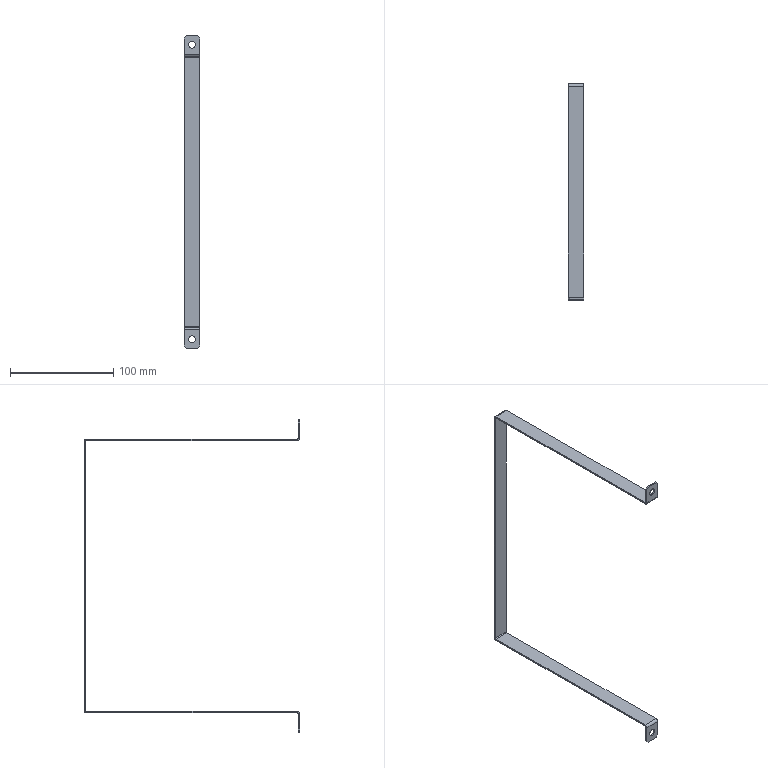Part | SolidWorks | features BaseBody 1 | 1 solid | 30 faces | box 15 x 208.5 x 302 mm | volume 15925 mm3 | plane 18 | cylinder 12 | commonest cylinder face diameters 1.473 x4 4.473 x4 7 x4
STEP:
#1=CARTESIAN_POINT('',(0.,1.5,-146.));
#2=VERTEX_POINT('',#1);
#3=CARTESIAN_POINT('',(0.,1.5,-139.));
#4=VERTEX_POINT('',#3);
#5=CARTESIAN_POINT('',(0.,1.5,-142.5));
#6=DIRECTION('',(0.,1.,0.));
#7=DIRECTION('',(0.,0.,-1.));
#8=AXIS2_PLACEMENT_3D('',#5,#6,#7);
#9=CIRCLE('',#8,3.5);
#10=EDGE_CURVE('',#2,#4,#9,.T.);
#11=ORIENTED_EDGE('',*,*,#10,.T.);
#12=CARTESIAN_POINT('',(0.,0.,-139.));
#13=VERTEX_POINT('',#12);
#14=CARTESIAN_POINT('',(0.,208.501,-139.));
#15=DIRECTION('',(0.,-1.,0.));
#16=VECTOR('',#15,1000.);
#17=LINE('',#14,#16);
#18=EDGE_CURVE('',#4,#13,#17,.T.);
#19=ORIENTED_EDGE('',*,*,#18,.T.);
#20=CARTESIAN_POINT('',(0.,0.,-146.));
#21=VERTEX_POINT('',#20);
#22=CARTESIAN_POINT('',(0.,0.,-142.5));
#23=DIRECTION('',(0.,-1.,0.));
#24=DIRECTION('',(0.,0.,1.));
#25=AXIS2_PLACEMENT_3D('',#22,#23,#24);
#26=CIRCLE('',#25,3.5);
#27=EDGE_CURVE('',#13,#21,#26,.T.);
#28=ORIENTED_EDGE('',*,*,#27,.T.);
#29=CARTESIAN_POINT('',(0.,208.501,-146.));
#30=DIRECTION('',(0.,-1.,0.));
#31=VECTOR('',#30,1000.);
#32=LINE('',#29,#31);
#33=EDGE_CURVE('',#2,#21,#32,.T.);
#34=ORIENTED_EDGE('',*,*,#33,.F.);
#35=EDGE_LOOP('',(#11,#19,#28,#34));
#36=FACE_OUTER_BOUND('',#35,.T.);
#37=CARTESIAN_POINT('',(0.,208.501,-142.5));
#38=DIRECTION('',(0.,-1.,0.));
#39=DIRECTION('',(0.,0.,-1.));
#40=AXIS2_PLACEMENT_3D('',#37,#38,#39);
#41=CYLINDRICAL_SURFACE('',#40,3.5);
#42=ADVANCED_FACE('',(#36),#41,.F.);
#43=CARTESIAN_POINT('',(0.,1.5,139.));
#44=VERTEX_POINT('',#43);
#45=CARTESIAN_POINT('',(0.,1.5,146.));
#46=VERTEX_POINT('',#45);
#47=CARTESIAN_POINT('',(0.,1.5,142.5));
#48=DIRECTION('',(0.,1.,0.));
#49=DIRECTION('',(0.,0.,-1.));
#50=AXIS2_PLACEMENT_3D('',#47,#48,#49);
#51=CIRCLE('',#50,3.5);
#52=EDGE_CURVE('',#44,#46,#51,.T.);
#53=ORIENTED_EDGE('',*,*,#52,.T.);
#54=CARTESIAN_POINT('',(0.,0.,146.));
#55=VERTEX_POINT('',#54);
#56=CARTESIAN_POINT('',(0.,208.501,146.));
#57=DIRECTION('',(0.,-1.,0.));
#58=VECTOR('',#57,1000.);
#59=LINE('',#56,#58);
#60=EDGE_CURVE('',#46,#55,#59,.T.);
#61=ORIENTED_EDGE('',*,*,#60,.T.);
#62=CARTESIAN_POINT('',(0.,0.,139.));
#63=VERTEX_POINT('',#62);
#64=CARTESIAN_POINT('',(0.,0.,142.5));
#65=DIRECTION('',(0.,-1.,0.));
#66=DIRECTION('',(0.,0.,-1.));
#67=AXIS2_PLACEMENT_3D('',#64,#65,#66);
#68=CIRCLE('',#67,3.5);
#69=EDGE_CURVE('',#55,#63,#68,.T.);
#70=ORIENTED_EDGE('',*,*,#69,.T.);
#71=CARTESIAN_POINT('',(0.,208.501,139.));
#72=DIRECTION('',(0.,-1.,0.));
#73=VECTOR('',#72,1000.);
#74=LINE('',#71,#73);
#75=EDGE_CURVE('',#44,#63,#74,.T.);
#76=ORIENTED_EDGE('',*,*,#75,.F.);
#77=EDGE_LOOP('',(#53,#61,#70,#76));
#78=FACE_OUTER_BOUND('',#77,.T.);
#79=CARTESIAN_POINT('',(0.,208.501,142.5));
#80=DIRECTION('',(0.,-1.,0.));
#81=DIRECTION('',(0.,0.,-1.));
#82=AXIS2_PLACEMENT_3D('',#79,#80,#81);
#83=CYLINDRICAL_SURFACE('',#82,3.5);
#84=ADVANCED_FACE('',(#78),#83,.F.);
#85=CARTESIAN_POINT('',(-5.5,0.,151.));
#86=VERTEX_POINT('',#85);
#87=CARTESIAN_POINT('',(-7.5,0.,149.));
#88=VERTEX_POINT('',#87);
#89=CARTESIAN_POINT('',(1.,0.,157.5));
#90=DIRECTION('',(-0.7071,0.,-0.7071));
#91=VECTOR('',#90,1000.);
#92=LINE('',#89,#91);
#93=EDGE_CURVE('',#86,#88,#92,.T.);
#94=ORIENTED_EDGE('',*,*,#93,.F.);
#95=CARTESIAN_POINT('',(-5.5,1.5,151.));
#96=VERTEX_POINT('',#95);
#97=CARTESIAN_POINT('',(-5.5,0.,151.));
#98=DIRECTION('',(0.,-1.,0.));
#99=VECTOR('',#98,1000.);
#100=LINE('',#97,#99);
#101=EDGE_CURVE('',#96,#86,#100,.T.);
#102=ORIENTED_EDGE('',*,*,#101,.F.);
#103=CARTESIAN_POINT('',(-7.5,1.5,149.));
#104=VERTEX_POINT('',#103);
#105=CARTESIAN_POINT('',(-7.5,1.5,149.));
#106=DIRECTION('',(0.7071,0.,0.7071));
#107=VECTOR('',#106,1000.);
#108=LINE('',#105,#107);
#109=EDGE_CURVE('',#104,#96,#108,.T.);
#110=ORIENTED_EDGE('',*,*,#109,.F.);
#111=CARTESIAN_POINT('',(-7.5,2.237,149.));
#112=DIRECTION('',(0.,1.,0.));
#113=VECTOR('',#112,1000.);
#114=LINE('',#111,#113);
#115=EDGE_CURVE('',#88,#104,#114,.T.);
#116=ORIENTED_EDGE('',*,*,#115,.F.);
#117=EDGE_LOOP('',(#94,#102,#110,#116));
#118=FACE_OUTER_BOUND('',#117,.T.);
#119=CARTESIAN_POINT('',(-7.5,2.237,149.));
#120=DIRECTION('',(0.7071,0.,-0.7071));
#121=DIRECTION('',(0.,-1.,0.));
#122=AXIS2_PLACEMENT_3D('',#119,#120,#121);
#123=PLANE('',#122);
#124=ADVANCED_FACE('',(#118),#123,.F.);
#125=CARTESIAN_POINT('',(7.5,0.,149.));
#126=VERTEX_POINT('',#125);
#127=CARTESIAN_POINT('',(5.5,0.,151.));
#128=VERTEX_POINT('',#127);
#129=CARTESIAN_POINT('',(6.5,0.,150.));
#130=DIRECTION('',(-0.7071,0.,0.7071));
#131=VECTOR('',#130,1000.);
#132=LINE('',#129,#131);
#133=EDGE_CURVE('',#126,#128,#132,.T.);
#134=ORIENTED_EDGE('',*,*,#133,.F.);
#135=CARTESIAN_POINT('',(7.5,1.5,149.));
#136=VERTEX_POINT('',#135);
#137=CARTESIAN_POINT('',(7.5,2.237,149.));
#138=DIRECTION('',(0.,-1.,0.));
#139=VECTOR('',#138,1000.);
#140=LINE('',#137,#139);
#141=EDGE_CURVE('',#136,#126,#140,.T.);
#142=ORIENTED_EDGE('',*,*,#141,.F.);
#143=CARTESIAN_POINT('',(5.5,1.5,151.));
#144=VERTEX_POINT('',#143);
#145=CARTESIAN_POINT('',(5.5,1.5,151.));
#146=DIRECTION('',(0.7071,0.,-0.7071));
#147=VECTOR('',#146,1000.);
#148=LINE('',#145,#147);
#149=EDGE_CURVE('',#144,#136,#148,.T.);
#150=ORIENTED_EDGE('',*,*,#149,.F.);
#151=CARTESIAN_POINT('',(5.5,0.,151.));
#152=DIRECTION('',(0.,1.,0.));
#153=VECTOR('',#152,1000.);
#154=LINE('',#151,#153);
#155=EDGE_CURVE('',#128,#144,#154,.T.);
#156=ORIENTED_EDGE('',*,*,#155,.F.);
#157=EDGE_LOOP('',(#134,#142,#150,#156));
#158=FACE_OUTER_BOUND('',#157,.T.);
#159=CARTESIAN_POINT('',(5.5,0.,151.));
#160=DIRECTION('',(-0.7071,0.,-0.7071));
#161=DIRECTION('',(-0.7071,0.,0.7071));
#162=AXIS2_PLACEMENT_3D('',#159,#160,#161);
#163=PLANE('',#162);
#164=ADVANCED_FACE('',(#158),#163,.F.);
#165=CARTESIAN_POINT('',(-5.5,1.5,-151.));
#166=VERTEX_POINT('',#165);
#167=CARTESIAN_POINT('',(-7.5,1.5,-149.));
#168=VERTEX_POINT('',#167);
#169=CARTESIAN_POINT('',(-7.5,1.5,-149.));
#170=DIRECTION('',(-0.7071,0.,0.7071));
#171=VECTOR('',#170,1000.);
#172=LINE('',#169,#171);
#173=EDGE_CURVE('',#166,#168,#172,.T.);
#174=ORIENTED_EDGE('',*,*,#173,.F.);
#175=CARTESIAN_POINT('',(-5.5,0.,-151.));
#176=VERTEX_POINT('',#175);
#177=CARTESIAN_POINT('',(-5.5,1.5,-151.));
#178=DIRECTION('',(0.,1.,0.));
#179=VECTOR('',#178,1000.);
#180=LINE('',#177,#179);
#181=EDGE_CURVE('',#176,#166,#180,.T.);
#182=ORIENTED_EDGE('',*,*,#181,.F.);
#183=CARTESIAN_POINT('',(-7.5,0.,-149.));
#184=VERTEX_POINT('',#183);
#185=CARTESIAN_POINT('',(1.,0.,-157.5));
#186=DIRECTION('',(0.7071,0.,-0.7071));
#187=VECTOR('',#186,1000.);
#188=LINE('',#185,#187);
#189=EDGE_CURVE('',#184,#176,#188,.T.);
#190=ORIENTED_EDGE('',*,*,#189,.F.);
#191=CARTESIAN_POINT('',(-7.5,2.237,-149.));
#192=DIRECTION('',(0.,-1.,0.));
#193=VECTOR('',#192,1000.);
#194=LINE('',#191,#193);
#195=EDGE_CURVE('',#168,#184,#194,.T.);
#196=ORIENTED_EDGE('',*,*,#195,.F.);
#197=EDGE_LOOP('',(#174,#182,#190,#196));
#198=FACE_OUTER_BOUND('',#197,.T.);
#199=CARTESIAN_POINT('',(-7.5,2.237,-149.));
#200=DIRECTION('',(0.7071,0.,0.7071));
#201=DIRECTION('',(0.,-1.,0.));
#202=AXIS2_PLACEMENT_3D('',#199,#200,#201);
#203=PLANE('',#202);
#204=ADVANCED_FACE('',(#198),#203,.F.);
#205=CARTESIAN_POINT('',(7.5,1.5,-149.));
#206=VERTEX_POINT('',#205);
#207=CARTESIAN_POINT('',(5.5,1.5,-151.));
#208=VERTEX_POINT('',#207);
#209=CARTESIAN_POINT('',(5.5,1.5,-151.));
#210=DIRECTION('',(-0.7071,0.,-0.7071));
#211=VECTOR('',#210,1000.);
#212=LINE('',#209,#211);
#213=EDGE_CURVE('',#206,#208,#212,.T.);
#214=ORIENTED_EDGE('',*,*,#213,.F.);
#215=CARTESIAN_POINT('',(7.5,0.,-149.));
#216=VERTEX_POINT('',#215);
#217=CARTESIAN_POINT('',(7.5,1.5,-149.));
#218=DIRECTION('',(0.,1.,0.));
#219=VECTOR('',#218,1000.);
#220=LINE('',#217,#219);
#221=EDGE_CURVE('',#216,#206,#220,.T.);
#222=ORIENTED_EDGE('',*,*,#221,.F.);
#223=CARTESIAN_POINT('',(5.5,0.,-151.));
#224=VERTEX_POINT('',#223);
#225=CARTESIAN_POINT('',(6.5,0.,-150.));
#226=DIRECTION('',(0.7071,0.,0.7071));
#227=VECTOR('',#226,1000.);
#228=LINE('',#225,#227);
#229=EDGE_CURVE('',#224,#216,#228,.T.);
#230=ORIENTED_EDGE('',*,*,#229,.F.);
#231=CARTESIAN_POINT('',(5.5,0.,-151.));
#232=DIRECTION('',(0.,-1.,0.));
#233=VECTOR('',#232,1000.);
#234=LINE('',#231,#233);
#235=EDGE_CURVE('',#208,#224,#234,.T.);
#236=ORIENTED_EDGE('',*,*,#235,.F.);
#237=EDGE_LOOP('',(#214,#222,#230,#236));
#238=FACE_OUTER_BOUND('',#237,.T.);
#239=CARTESIAN_POINT('',(5.5,1.5,-151.));
#240=DIRECTION('',(0.7071,0.,-0.7071));
#241=DIRECTION('',(0.,-1.,0.));
#242=AXIS2_PLACEMENT_3D('',#239,#240,#241);
#243=PLANE('',#242);
#244=ADVANCED_FACE('',(#238),#243,.T.);
#245=CARTESIAN_POINT('',(-7.5,2.237,132.5));
#246=VERTEX_POINT('',#245);
#247=CARTESIAN_POINT('',(-7.5,1.5,133.237));
#248=VERTEX_POINT('',#247);
#249=CARTESIAN_POINT('',(-7.5,2.237,133.237));
#250=DIRECTION('',(-1.,0.,0.));
#251=DIRECTION('',(0.,0.,-1.));
#252=AXIS2_PLACEMENT_3D('',#249,#250,#251);
#253=CIRCLE('',#252,0.7366);
#254=EDGE_CURVE('',#246,#248,#253,.T.);
#255=ORIENTED_EDGE('',*,*,#254,.T.);
#256=CARTESIAN_POINT('',(7.5,1.5,133.237));
#257=VERTEX_POINT('',#256);
#258=CARTESIAN_POINT('',(7.5,1.5,133.237));
#259=DIRECTION('',(-1.,0.,0.));
#260=VECTOR('',#259,1000.);
#261=LINE('',#258,#260);
#262=EDGE_CURVE('',#257,#248,#261,.T.);
#263=ORIENTED_EDGE('',*,*,#262,.F.);
#264=CARTESIAN_POINT('',(7.5,2.237,132.5));
#265=VERTEX_POINT('',#264);
#266=CARTESIAN_POINT('',(7.5,2.237,133.237));
#267=DIRECTION('',(-1.,0.,0.));
#268=DIRECTION('',(0.,0.,-1.));
#269=AXIS2_PLACEMENT_3D('',#266,#267,#268);
#270=CIRCLE('',#269,0.7366);
#271=EDGE_CURVE('',#265,#257,#270,.T.);
#272=ORIENTED_EDGE('',*,*,#271,.F.);
#273=CARTESIAN_POINT('',(7.5,2.237,132.5));
#274=DIRECTION('',(-1.,0.,0.));
#275=VECTOR('',#274,1000.);
#276=LINE('',#273,#275);
#277=EDGE_CURVE('',#265,#246,#276,.T.);
#278=ORIENTED_EDGE('',*,*,#277,.T.);
#279=EDGE_LOOP('',(#255,#263,#272,#278));
#280=FACE_OUTER_BOUND('',#279,.T.);
#281=CARTESIAN_POINT('',(7.5,2.237,133.237));
#282=DIRECTION('',(-1.,0.,0.));
#283=DIRECTION('',(0.,0.,1.));
#284=AXIS2_PLACEMENT_3D('',#281,#282,#283);
#285=CYLINDRICAL_SURFACE('',#284,0.7366);
#286=ADVANCED_FACE('',(#280),#285,.F.);
#287=CARTESIAN_POINT('',(-7.5,206.263,132.5));
#288=VERTEX_POINT('',#287);
#289=CARTESIAN_POINT('',(-7.5,0.,132.5));
#290=DIRECTION('',(0.,-1.,0.));
#291=VECTOR('',#290,1000.);
#292=LINE('',#289,#291);
#293=EDGE_CURVE('',#288,#246,#292,.T.);
#294=ORIENTED_EDGE('',*,*,#293,.T.);
#295=ORIENTED_EDGE('',*,*,#277,.F.);
#296=CARTESIAN_POINT('',(7.5,206.263,132.5));
#297=VERTEX_POINT('',#296);
#298=CARTESIAN_POINT('',(7.5,0.,132.5));
#299=DIRECTION('',(0.,-1.,0.));
#300=VECTOR('',#299,1000.);
#301=LINE('',#298,#300);
#302=EDGE_CURVE('',#297,#265,#301,.T.);
#303=ORIENTED_EDGE('',*,*,#302,.F.);
#304=CARTESIAN_POINT('',(7.5,206.263,132.5));
#305=DIRECTION('',(-1.,0.,0.));
#306=VECTOR('',#305,1000.);
#307=LINE('',#304,#306);
#308=EDGE_CURVE('',#297,#288,#307,.T.);
#309=ORIENTED_EDGE('',*,*,#308,.T.);
#310=EDGE_LOOP('',(#294,#295,#303,#309));
#311=FACE_OUTER_BOUND('',#310,.T.);
#312=CARTESIAN_POINT('',(7.5,0.,132.5));
#313=DIRECTION('',(0.,0.,-1.));
#314=DIRECTION('',(0.,-1.,0.));
#315=AXIS2_PLACEMENT_3D('',#312,#313,#314);
#316=PLANE('',#315);
#317=ADVANCED_FACE('',(#311),#316,.F.);
#318=CARTESIAN_POINT('',(-7.5,208.5,130.263));
#319=VERTEX_POINT('',#318);
#320=CARTESIAN_POINT('',(-7.5,206.263,130.263));
#321=DIRECTION('',(1.,0.,0.));
#322=DIRECTION('',(0.,0.,-1.));
#323=AXIS2_PLACEMENT_3D('',#320,#321,#322);
#324=CIRCLE('',#323,2.237);
#325=EDGE_CURVE('',#319,#288,#324,.T.);
#326=ORIENTED_EDGE('',*,*,#325,.T.);
#327=ORIENTED_EDGE('',*,*,#308,.F.);
#328=CARTESIAN_POINT('',(7.5,208.5,130.263));
#329=VERTEX_POINT('',#328);
#330=CARTESIAN_POINT('',(7.5,206.263,130.263));
#331=DIRECTION('',(1.,0.,0.));
#332=DIRECTION('',(0.,0.,-1.));
#333=AXIS2_PLACEMENT_3D('',#330,#331,#332);
#334=CIRCLE('',#333,2.237);
#335=EDGE_CURVE('',#329,#297,#334,.T.);
#336=ORIENTED_EDGE('',*,*,#335,.F.);
#337=CARTESIAN_POINT('',(7.5,208.5,130.263));
#338=DIRECTION('',(-1.,0.,0.));
#339=VECTOR('',#338,1000.);
#340=LINE('',#337,#339);
#341=EDGE_CURVE('',#329,#319,#340,.T.);
#342=ORIENTED_EDGE('',*,*,#341,.T.);
#343=EDGE_LOOP('',(#326,#327,#336,#342));
#344=FACE_OUTER_BOUND('',#343,.T.);
#345=CARTESIAN_POINT('',(7.5,206.263,130.263));
#346=DIRECTION('',(-1.,0.,0.));
#347=DIRECTION('',(0.,0.,1.));
#348=AXIS2_PLACEMENT_3D('',#345,#346,#347);
#349=CYLINDRICAL_SURFACE('',#348,2.237);
#350=ADVANCED_FACE('',(#344),#349,.T.);
#351=CARTESIAN_POINT('',(-7.5,208.5,-130.263));
#352=VERTEX_POINT('',#351);
#353=CARTESIAN_POINT('',(-7.5,208.5,131.));
#354=DIRECTION('',(0.,0.,1.));
#355=VECTOR('',#354,1000.);
#356=LINE('',#353,#355);
#357=EDGE_CURVE('',#352,#319,#356,.T.);
#358=ORIENTED_EDGE('',*,*,#357,.T.);
#359=ORIENTED_EDGE('',*,*,#341,.F.);
#360=CARTESIAN_POINT('',(7.5,208.5,-130.263));
#361=VERTEX_POINT('',#360);
#362=CARTESIAN_POINT('',(7.5,208.5,131.));
#363=DIRECTION('',(0.,0.,1.));
#364=VECTOR('',#363,1000.);
#365=LINE('',#362,#364);
#366=EDGE_CURVE('',#361,#329,#365,.T.);
#367=ORIENTED_EDGE('',*,*,#366,.F.);
#368=CARTESIAN_POINT('',(7.5,208.5,-130.263));
#369=DIRECTION('',(-1.,0.,0.));
#370=VECTOR('',#369,1000.);
#371=LINE('',#368,#370);
#372=EDGE_CURVE('',#361,#352,#371,.T.);
#373=ORIENTED_EDGE('',*,*,#372,.T.);
#374=EDGE_LOOP('',(#358,#359,#367,#373));
#375=FACE_OUTER_BOUND('',#374,.T.);
#376=CARTESIAN_POINT('',(7.5,208.5,131.));
#377=DIRECTION('',(0.,-1.,0.));
#378=DIRECTION('',(0.,0.,-1.));
#379=AXIS2_PLACEMENT_3D('',#376,#377,#378);
#380=PLANE('',#379);
#381=ADVANCED_FACE('',(#375),#380,.F.);
#382=CARTESIAN_POINT('',(-7.5,206.263,-132.5));
#383=VERTEX_POINT('',#382);
#384=CARTESIAN_POINT('',(-7.5,206.263,-130.263));
#385=DIRECTION('',(1.,0.,0.));
#386=DIRECTION('',(0.,0.,-1.));
#387=AXIS2_PLACEMENT_3D('',#384,#385,#386);
#388=CIRCLE('',#387,2.237);
#389=EDGE_CURVE('',#383,#352,#388,.T.);
#390=ORIENTED_EDGE('',*,*,#389,.T.);
#391=ORIENTED_EDGE('',*,*,#372,.F.);
#392=CARTESIAN_POINT('',(7.5,206.263,-132.5));
#393=VERTEX_POINT('',#392);
#394=CARTESIAN_POINT('',(7.5,206.263,-130.263));
#395=DIRECTION('',(1.,0.,0.));
#396=DIRECTION('',(0.,0.,-1.));
#397=AXIS2_PLACEMENT_3D('',#394,#395,#396);
#398=CIRCLE('',#397,2.237);
#399=EDGE_CURVE('',#393,#361,#398,.T.);
#400=ORIENTED_EDGE('',*,*,#399,.F.);
#401=CARTESIAN_POINT('',(7.5,206.263,-132.5));
#402=DIRECTION('',(-1.,0.,0.));
#403=VECTOR('',#402,1000.);
#404=LINE('',#401,#403);
#405=EDGE_CURVE('',#393,#383,#404,.T.);
#406=ORIENTED_EDGE('',*,*,#405,.T.);
#407=EDGE_LOOP('',(#390,#391,#400,#406));
#408=FACE_OUTER_BOUND('',#407,.T.);
#409=CARTESIAN_POINT('',(7.5,206.263,-130.263));
#410=DIRECTION('',(-1.,0.,0.));
#411=DIRECTION('',(0.,0.,1.));
#412=AXIS2_PLACEMENT_3D('',#409,#410,#411);
#413=CYLINDRICAL_SURFACE('',#412,2.237);
#414=ADVANCED_FACE('',(#408),#413,.T.);
#415=CARTESIAN_POINT('',(-7.5,2.237,-132.5));
#416=VERTEX_POINT('',#415);
#417=CARTESIAN_POINT('',(-7.5,0.,-132.5));
#418=DIRECTION('',(0.,1.,0.));
#419=VECTOR('',#418,1000.);
#420=LINE('',#417,#419);
#421=EDGE_CURVE('',#416,#383,#420,.T.);
#422=ORIENTED_EDGE('',*,*,#421,.T.);
#423=ORIENTED_EDGE('',*,*,#405,.F.);
#424=CARTESIAN_POINT('',(7.5,2.237,-132.5));
#425=VERTEX_POINT('',#424);
#426=CARTESIAN_POINT('',(7.5,0.,-132.5));
#427=DIRECTION('',(0.,1.,0.));
#428=VECTOR('',#427,1000.);
#429=LINE('',#426,#428);
#430=EDGE_CURVE('',#425,#393,#429,.T.);
#431=ORIENTED_EDGE('',*,*,#430,.F.);
#432=CARTESIAN_POINT('',(7.5,2.237,-132.5));
#433=DIRECTION('',(-1.,0.,0.));
#434=VECTOR('',#433,1000.);
#435=LINE('',#432,#434);
#436=EDGE_CURVE('',#425,#416,#435,.T.);
#437=ORIENTED_EDGE('',*,*,#436,.T.);
#438=EDGE_LOOP('',(#422,#423,#431,#437));
#439=FACE_OUTER_BOUND('',#438,.T.);
#440=CARTESIAN_POINT('',(7.5,0.,-132.5));
#441=DIRECTION('',(0.,0.,1.));
#442=DIRECTION('',(0.,-1.,0.));
#443=AXIS2_PLACEMENT_3D('',#440,#441,#442);
#444=PLANE('',#443);
#445=ADVANCED_FACE('',(#439),#444,.F.);
#446=CARTESIAN_POINT('',(-7.5,1.5,-133.237));
#447=VERTEX_POINT('',#446);
#448=CARTESIAN_POINT('',(-7.5,2.237,-133.237));
#449=DIRECTION('',(-1.,0.,0.));
#450=DIRECTION('',(0.,0.,-1.));
#451=AXIS2_PLACEMENT_3D('',#448,#449,#450);
#452=CIRCLE('',#451,0.7366);
#453=EDGE_CURVE('',#447,#416,#452,.T.);
#454=ORIENTED_EDGE('',*,*,#453,.T.);
#455=ORIENTED_EDGE('',*,*,#436,.F.);
#456=CARTESIAN_POINT('',(7.5,1.5,-133.237));
#457=VERTEX_POINT('',#456);
#458=CARTESIAN_POINT('',(7.5,2.237,-133.237));
#459=DIRECTION('',(-1.,0.,0.));
#460=DIRECTION('',(0.,0.,-1.));
#461=AXIS2_PLACEMENT_3D('',#458,#459,#460);
#462=CIRCLE('',#461,0.7366);
#463=EDGE_CURVE('',#457,#425,#462,.T.);
#464=ORIENTED_EDGE('',*,*,#463,.F.);
#465=CARTESIAN_POINT('',(7.5,1.5,-133.237));
#466=DIRECTION('',(-1.,0.,0.));
#467=VECTOR('',#466,1000.);
#468=LINE('',#465,#467);
#469=EDGE_CURVE('',#457,#447,#468,.T.);
#470=ORIENTED_EDGE('',*,*,#469,.T.);
#471=EDGE_LOOP('',(#454,#455,#464,#470));
#472=FACE_OUTER_BOUND('',#471,.T.);
#473=CARTESIAN_POINT('',(7.5,2.237,-133.237));
#474=DIRECTION('',(-1.,0.,0.));
#475=DIRECTION('',(0.,0.,1.));
#476=AXIS2_PLACEMENT_3D('',#473,#474,#475);
#477=CYLINDRICAL_SURFACE('',#476,0.7366);
#478=ADVANCED_FACE('',(#472),#477,.F.);
#479=ORIENTED_EDGE('',*,*,#10,.F.);
#480=CARTESIAN_POINT('',(0.,1.5,-142.5));
#481=DIRECTION('',(0.,1.,0.));
#482=DIRECTION('',(0.,0.,-1.));
#483=AXIS2_PLACEMENT_3D('',#480,#481,#482);
#484=CIRCLE('',#483,3.5);
#485=EDGE_CURVE('',#4,#2,#484,.T.);
#486=ORIENTED_EDGE('',*,*,#485,.F.);
#487=EDGE_LOOP('',(#479,#486));
#488=FACE_BOUND('',#487,.T.);
#489=CARTESIAN_POINT('',(7.5,1.5,-151.));
#490=DIRECTION('',(0.,0.,1.));
#491=VECTOR('',#490,1000.);
#492=LINE('',#489,#491);
#493=EDGE_CURVE('',#206,#457,#492,.T.);
#494=ORIENTED_EDGE('',*,*,#493,.F.);
#495=ORIENTED_EDGE('',*,*,#213,.T.);
#496=CARTESIAN_POINT('',(7.5,1.5,-151.));
#497=DIRECTION('',(-1.,0.,0.));
#498=VECTOR('',#497,1000.);
#499=LINE('',#496,#498);
#500=EDGE_CURVE('',#208,#166,#499,.T.);
#501=ORIENTED_EDGE('',*,*,#500,.T.);
#502=ORIENTED_EDGE('',*,*,#173,.T.);
#503=CARTESIAN_POINT('',(-7.5,1.5,-151.));
#504=DIRECTION('',(0.,0.,1.));
#505=VECTOR('',#504,1000.);
#506=LINE('',#503,#505);
#507=EDGE_CURVE('',#168,#447,#506,.T.);
#508=ORIENTED_EDGE('',*,*,#507,.T.);
#509=ORIENTED_EDGE('',*,*,#469,.F.);
#510=EDGE_LOOP('',(#494,#495,#501,#502,#508,#509));
#511=FACE_OUTER_BOUND('',#510,.T.);
#512=CARTESIAN_POINT('',(7.5,1.5,-151.));
#513=DIRECTION('',(0.,-1.,0.));
#514=DIRECTION('',(0.,0.,-1.));
#515=AXIS2_PLACEMENT_3D('',#512,#513,#514);
#516=PLANE('',#515);
#517=ADVANCED_FACE('',(#488,#511),#516,.F.);
#518=ORIENTED_EDGE('',*,*,#500,.F.);
#519=ORIENTED_EDGE('',*,*,#235,.T.);
#520=CARTESIAN_POINT('',(7.5,0.,-151.));
#521=DIRECTION('',(-1.,0.,0.));
#522=VECTOR('',#521,1000.);
#523=LINE('',#520,#522);
#524=EDGE_CURVE('',#224,#176,#523,.T.);
#525=ORIENTED_EDGE('',*,*,#524,.T.);
#526=ORIENTED_EDGE('',*,*,#181,.T.);
#527=EDGE_LOOP('',(#518,#519,#525,#526));
#528=FACE_OUTER_BOUND('',#527,.T.);
#529=CARTESIAN_POINT('',(7.5,1.5,-151.));
#530=DIRECTION('',(0.,0.,-1.));
#531=DIRECTION('',(0.,-1.,0.));
#532=AXIS2_PLACEMENT_3D('',#529,#530,#531);
#533=PLANE('',#532);
#534=ADVANCED_FACE('',(#528),#533,.T.);
#535=CARTESIAN_POINT('',(0.,0.,-142.5));
#536=DIRECTION('',(0.,-1.,0.));
#537=DIRECTION('',(0.,0.,1.));
#538=AXIS2_PLACEMENT_3D('',#535,#536,#537);
#539=CIRCLE('',#538,3.5);
#540=EDGE_CURVE('',#21,#13,#539,.T.);
#541=ORIENTED_EDGE('',*,*,#540,.F.);
#542=ORIENTED_EDGE('',*,*,#27,.F.);
#543=EDGE_LOOP('',(#541,#542));
#544=FACE_BOUND('',#543,.T.);
#545=ORIENTED_EDGE('',*,*,#524,.F.);
#546=ORIENTED_EDGE('',*,*,#229,.T.);
#547=CARTESIAN_POINT('',(7.5,0.,-133.237));
#548=VERTEX_POINT('',#547);
#549=CARTESIAN_POINT('',(7.5,0.,-151.));
#550=DIRECTION('',(0.,0.,1.));
#551=VECTOR('',#550,1000.);
#552=LINE('',#549,#551);
#553=EDGE_CURVE('',#216,#548,#552,.T.);
#554=ORIENTED_EDGE('',*,*,#553,.T.);
#555=CARTESIAN_POINT('',(-7.5,0.,-133.237));
#556=VERTEX_POINT('',#555);
#557=CARTESIAN_POINT('',(7.5,0.,-133.237));
#558=DIRECTION('',(-1.,0.,0.));
#559=VECTOR('',#558,1000.);
#560=LINE('',#557,#559);
#561=EDGE_CURVE('',#548,#556,#560,.T.);
#562=ORIENTED_EDGE('',*,*,#561,.T.);
#563=CARTESIAN_POINT('',(-7.5,0.,-151.));
#564=DIRECTION('',(0.,0.,1.));
#565=VECTOR('',#564,1000.);
#566=LINE('',#563,#565);
#567=EDGE_CURVE('',#184,#556,#566,.T.);
#568=ORIENTED_EDGE('',*,*,#567,.F.);
#569=ORIENTED_EDGE('',*,*,#189,.T.);
#570=EDGE_LOOP('',(#545,#546,#554,#562,#568,#569));
#571=FACE_OUTER_BOUND('',#570,.T.);
#572=CARTESIAN_POINT('',(7.5,0.,-151.));
#573=DIRECTION('',(0.,-1.,0.));
#574=DIRECTION('',(0.,0.,-1.));
#575=AXIS2_PLACEMENT_3D('',#572,#573,#574);
#576=PLANE('',#575);
#577=ADVANCED_FACE('',(#544,#571),#576,.T.);
#578=CARTESIAN_POINT('',(-7.5,2.237,-131.));
#579=VERTEX_POINT('',#578);
#580=CARTESIAN_POINT('',(-7.5,2.237,-133.237));
#581=DIRECTION('',(-1.,0.,0.));
#582=DIRECTION('',(0.,0.,1.));
#583=AXIS2_PLACEMENT_3D('',#580,#581,#582);
#584=CIRCLE('',#583,2.237);
#585=EDGE_CURVE('',#556,#579,#584,.T.);
#586=ORIENTED_EDGE('',*,*,#585,.F.);
#587=ORIENTED_EDGE('',*,*,#561,.F.);
#588=CARTESIAN_POINT('',(7.5,2.237,-131.));
#589=VERTEX_POINT('',#588);
#590=CARTESIAN_POINT('',(7.5,2.237,-133.237));
#591=DIRECTION('',(-1.,0.,0.));
#592=DIRECTION('',(0.,0.,1.));
#593=AXIS2_PLACEMENT_3D('',#590,#591,#592);
#594=CIRCLE('',#593,2.237);
#595=EDGE_CURVE('',#548,#589,#594,.T.);
#596=ORIENTED_EDGE('',*,*,#595,.T.);
#597=CARTESIAN_POINT('',(7.5,2.237,-131.));
#598=DIRECTION('',(-1.,0.,0.));
#599=VECTOR('',#598,1000.);
#600=LINE('',#597,#599);
#601=EDGE_CURVE('',#589,#579,#600,.T.);
#602=ORIENTED_EDGE('',*,*,#601,.T.);
#603=EDGE_LOOP('',(#586,#587,#596,#602));
#604=FACE_OUTER_BOUND('',#603,.T.);
#605=CARTESIAN_POINT('',(7.5,2.237,-133.237));
#606=DIRECTION('',(-1.,0.,0.));
#607=DIRECTION('',(0.,0.,1.));
#608=AXIS2_PLACEMENT_3D('',#605,#606,#607);
#609=CYLINDRICAL_SURFACE('',#608,2.237);
#610=ADVANCED_FACE('',(#604),#609,.T.);
#611=CARTESIAN_POINT('',(-7.5,206.263,-131.));
#612=VERTEX_POINT('',#611);
#613=CARTESIAN_POINT('',(-7.5,0.,-131.));
#614=DIRECTION('',(0.,1.,0.));
#615=VECTOR('',#614,1000.);
#616=LINE('',#613,#615);
#617=EDGE_CURVE('',#579,#612,#616,.T.);
#618=ORIENTED_EDGE('',*,*,#617,.F.);
#619=ORIENTED_EDGE('',*,*,#601,.F.);
#620=CARTESIAN_POINT('',(7.5,206.263,-131.));
#621=VERTEX_POINT('',#620);
#622=CARTESIAN_POINT('',(7.5,0.,-131.));
#623=DIRECTION('',(0.,1.,0.));
#624=VECTOR('',#623,1000.);
#625=LINE('',#622,#624);
#626=EDGE_CURVE('',#589,#621,#625,.T.);
#627=ORIENTED_EDGE('',*,*,#626,.T.);
#628=CARTESIAN_POINT('',(7.5,206.263,-131.));
#629=DIRECTION('',(-1.,0.,0.));
#630=VECTOR('',#629,1000.);
#631=LINE('',#628,#630);
#632=EDGE_CURVE('',#621,#612,#631,.T.);
#633=ORIENTED_EDGE('',*,*,#632,.T.);
#634=EDGE_LOOP('',(#618,#619,#627,#633));
#635=FACE_OUTER_BOUND('',#634,.T.);
#636=CARTESIAN_POINT('',(7.5,0.,-131.));
#637=DIRECTION('',(0.,0.,1.));
#638=DIRECTION('',(0.,-1.,0.));
#639=AXIS2_PLACEMENT_3D('',#636,#637,#638);
#640=PLANE('',#639);
#641=ADVANCED_FACE('',(#635),#640,.T.);
#642=CARTESIAN_POINT('',(-7.5,207.,-130.263));
#643=VERTEX_POINT('',#642);
#644=CARTESIAN_POINT('',(-7.5,206.263,-130.263));
#645=DIRECTION('',(1.,0.,0.));
#646=DIRECTION('',(0.,0.,-1.));
#647=AXIS2_PLACEMENT_3D('',#644,#645,#646);
#648=CIRCLE('',#647,0.7366);
#649=EDGE_CURVE('',#612,#643,#648,.T.);
#650=ORIENTED_EDGE('',*,*,#649,.F.);
#651=ORIENTED_EDGE('',*,*,#632,.F.);
#652=CARTESIAN_POINT('',(7.5,207.,-130.263));
#653=VERTEX_POINT('',#652);
#654=CARTESIAN_POINT('',(7.5,206.263,-130.263));
#655=DIRECTION('',(1.,0.,0.));
#656=DIRECTION('',(0.,0.,-1.));
#657=AXIS2_PLACEMENT_3D('',#654,#655,#656);
#658=CIRCLE('',#657,0.7366);
#659=EDGE_CURVE('',#621,#653,#658,.T.);
#660=ORIENTED_EDGE('',*,*,#659,.T.);
#661=CARTESIAN_POINT('',(7.5,207.,-130.263));
#662=DIRECTION('',(-1.,0.,0.));
#663=VECTOR('',#662,1000.);
#664=LINE('',#661,#663);
#665=EDGE_CURVE('',#653,#643,#664,.T.);
#666=ORIENTED_EDGE('',*,*,#665,.T.);
#667=EDGE_LOOP('',(#650,#651,#660,#666));
#668=FACE_OUTER_BOUND('',#667,.T.);
#669=CARTESIAN_POINT('',(7.5,206.263,-130.263));
#670=DIRECTION('',(-1.,0.,0.));
#671=DIRECTION('',(0.,0.,1.));
#672=AXIS2_PLACEMENT_3D('',#669,#670,#671);
#673=CYLINDRICAL_SURFACE('',#672,0.7366);
#674=ADVANCED_FACE('',(#668),#673,.F.);
#675=CARTESIAN_POINT('',(-7.5,207.,130.263));
#676=VERTEX_POINT('',#675);
#677=CARTESIAN_POINT('',(-7.5,207.,131.));
#678=DIRECTION('',(0.,0.,1.));
#679=VECTOR('',#678,1000.);
#680=LINE('',#677,#679);
#681=EDGE_CURVE('',#643,#676,#680,.T.);
#682=ORIENTED_EDGE('',*,*,#681,.F.);
#683=ORIENTED_EDGE('',*,*,#665,.F.);
#684=CARTESIAN_POINT('',(7.5,207.,130.263));
#685=VERTEX_POINT('',#684);
#686=CARTESIAN_POINT('',(7.5,207.,131.));
#687=DIRECTION('',(0.,0.,1.));
#688=VECTOR('',#687,1000.);
#689=LINE('',#686,#688);
#690=EDGE_CURVE('',#653,#685,#689,.T.);
#691=ORIENTED_EDGE('',*,*,#690,.T.);
#692=CARTESIAN_POINT('',(7.5,207.,130.263));
#693=DIRECTION('',(-1.,0.,0.));
#694=VECTOR('',#693,1000.);
#695=LINE('',#692,#694);
#696=EDGE_CURVE('',#685,#676,#695,.T.);
#697=ORIENTED_EDGE('',*,*,#696,.T.);
#698=EDGE_LOOP('',(#682,#683,#691,#697));
#699=FACE_OUTER_BOUND('',#698,.T.);
#700=CARTESIAN_POINT('',(7.5,207.,131.));
#701=DIRECTION('',(0.,-1.,0.));
#702=DIRECTION('',(0.,0.,-1.));
#703=AXIS2_PLACEMENT_3D('',#700,#701,#702);
#704=PLANE('',#703);
#705=ADVANCED_FACE('',(#699),#704,.T.);
#706=CARTESIAN_POINT('',(-7.5,206.263,131.));
#707=VERTEX_POINT('',#706);
#708=CARTESIAN_POINT('',(-7.5,206.263,130.263));
#709=DIRECTION('',(1.,0.,0.));
#710=DIRECTION('',(0.,0.,-1.));
#711=AXIS2_PLACEMENT_3D('',#708,#709,#710);
#712=CIRCLE('',#711,0.7366);
#713=EDGE_CURVE('',#676,#707,#712,.T.);
#714=ORIENTED_EDGE('',*,*,#713,.F.);
#715=ORIENTED_EDGE('',*,*,#696,.F.);
#716=CARTESIAN_POINT('',(7.5,206.263,131.));
#717=VERTEX_POINT('',#716);
#718=CARTESIAN_POINT('',(7.5,206.263,130.263));
#719=DIRECTION('',(1.,0.,0.));
#720=DIRECTION('',(0.,0.,-1.));
#721=AXIS2_PLACEMENT_3D('',#718,#719,#720);
#722=CIRCLE('',#721,0.7366);
#723=EDGE_CURVE('',#685,#717,#722,.T.);
#724=ORIENTED_EDGE('',*,*,#723,.T.);
#725=CARTESIAN_POINT('',(7.5,206.263,131.));
#726=DIRECTION('',(-1.,0.,0.));
#727=VECTOR('',#726,1000.);
#728=LINE('',#725,#727);
#729=EDGE_CURVE('',#717,#707,#728,.T.);
#730=ORIENTED_EDGE('',*,*,#729,.T.);
#731=EDGE_LOOP('',(#714,#715,#724,#730));
#732=FACE_OUTER_BOUND('',#731,.T.);
#733=CARTESIAN_POINT('',(7.5,206.263,130.263));
#734=DIRECTION('',(-1.,0.,0.));
#735=DIRECTION('',(0.,0.,1.));
#736=AXIS2_PLACEMENT_3D('',#733,#734,#735);
#737=CYLINDRICAL_SURFACE('',#736,0.7366);
#738=ADVANCED_FACE('',(#732),#737,.F.);
#739=CARTESIAN_POINT('',(-7.5,2.237,131.));
#740=VERTEX_POINT('',#739);
#741=CARTESIAN_POINT('',(-7.5,0.,131.));
#742=DIRECTION('',(0.,-1.,0.));
#743=VECTOR('',#742,1000.);
#744=LINE('',#741,#743);
#745=EDGE_CURVE('',#707,#740,#744,.T.);
#746=ORIENTED_EDGE('',*,*,#745,.F.);
#747=ORIENTED_EDGE('',*,*,#729,.F.);
#748=CARTESIAN_POINT('',(7.5,2.237,131.));
#749=VERTEX_POINT('',#748);
#750=CARTESIAN_POINT('',(7.5,0.,131.));
#751=DIRECTION('',(0.,-1.,0.));
#752=VECTOR('',#751,1000.);
#753=LINE('',#750,#752);
#754=EDGE_CURVE('',#717,#749,#753,.T.);
#755=ORIENTED_EDGE('',*,*,#754,.T.);
#756=CARTESIAN_POINT('',(7.5,2.237,131.));
#757=DIRECTION('',(-1.,0.,0.));
#758=VECTOR('',#757,1000.);
#759=LINE('',#756,#758);
#760=EDGE_CURVE('',#749,#740,#759,.T.);
#761=ORIENTED_EDGE('',*,*,#760,.T.);
#762=EDGE_LOOP('',(#746,#747,#755,#761));
#763=FACE_OUTER_BOUND('',#762,.T.);
#764=CARTESIAN_POINT('',(7.5,0.,131.));
#765=DIRECTION('',(0.,0.,-1.));
#766=DIRECTION('',(0.,-1.,0.));
#767=AXIS2_PLACEMENT_3D('',#764,#765,#766);
#768=PLANE('',#767);
#769=ADVANCED_FACE('',(#763),#768,.T.);
#770=CARTESIAN_POINT('',(-7.5,0.,133.237));
#771=VERTEX_POINT('',#770);
#772=CARTESIAN_POINT('',(-7.5,2.237,133.237));
#773=DIRECTION('',(-1.,0.,0.));
#774=DIRECTION('',(0.,0.,1.));
#775=AXIS2_PLACEMENT_3D('',#772,#773,#774);
#776=CIRCLE('',#775,2.237);
#777=EDGE_CURVE('',#740,#771,#776,.T.);
#778=ORIENTED_EDGE('',*,*,#777,.F.);
#779=ORIENTED_EDGE('',*,*,#760,.F.);
#780=CARTESIAN_POINT('',(7.5,0.,133.237));
#781=VERTEX_POINT('',#780);
#782=CARTESIAN_POINT('',(7.5,2.237,133.237));
#783=DIRECTION('',(-1.,0.,0.));
#784=DIRECTION('',(0.,0.,1.));
#785=AXIS2_PLACEMENT_3D('',#782,#783,#784);
#786=CIRCLE('',#785,2.237);
#787=EDGE_CURVE('',#749,#781,#786,.T.);
#788=ORIENTED_EDGE('',*,*,#787,.T.);
#789=CARTESIAN_POINT('',(7.5,0.,133.237));
#790=DIRECTION('',(-1.,0.,0.));
#791=VECTOR('',#790,1000.);
#792=LINE('',#789,#791);
#793=EDGE_CURVE('',#781,#771,#792,.T.);
#794=ORIENTED_EDGE('',*,*,#793,.T.);
#795=EDGE_LOOP('',(#778,#779,#788,#794));
#796=FACE_OUTER_BOUND('',#795,.T.);
#797=CARTESIAN_POINT('',(7.5,2.237,133.237));
#798=DIRECTION('',(-1.,0.,0.));
#799=DIRECTION('',(0.,0.,1.));
#800=AXIS2_PLACEMENT_3D('',#797,#798,#799);
#801=CYLINDRICAL_SURFACE('',#800,2.237);
#802=ADVANCED_FACE('',(#796),#801,.T.);
#803=CARTESIAN_POINT('',(0.,0.,142.5));
#804=DIRECTION('',(0.,-1.,0.));
#805=DIRECTION('',(0.,0.,-1.));
#806=AXIS2_PLACEMENT_3D('',#803,#804,#805);
#807=CIRCLE('',#806,3.5);
#808=EDGE_CURVE('',#63,#55,#807,.T.);
#809=ORIENTED_EDGE('',*,*,#808,.F.);
#810=ORIENTED_EDGE('',*,*,#69,.F.);
#811=EDGE_LOOP('',(#809,#810));
#812=FACE_BOUND('',#811,.T.);
#813=CARTESIAN_POINT('',(7.5,0.,151.));
#814=DIRECTION('',(0.,0.,1.));
#815=VECTOR('',#814,1000.);
#816=LINE('',#813,#815);
#817=EDGE_CURVE('',#781,#126,#816,.T.);
#818=ORIENTED_EDGE('',*,*,#817,.T.);
#819=ORIENTED_EDGE('',*,*,#133,.T.);
#820=CARTESIAN_POINT('',(7.5,0.,151.));
#821=DIRECTION('',(-1.,0.,0.));
#822=VECTOR('',#821,1000.);
#823=LINE('',#820,#822);
#824=EDGE_CURVE('',#128,#86,#823,.T.);
#825=ORIENTED_EDGE('',*,*,#824,.T.);
#826=ORIENTED_EDGE('',*,*,#93,.T.);
#827=CARTESIAN_POINT('',(-7.5,0.,151.));
#828=DIRECTION('',(0.,0.,1.));
#829=VECTOR('',#828,1000.);
#830=LINE('',#827,#829);
#831=EDGE_CURVE('',#771,#88,#830,.T.);
#832=ORIENTED_EDGE('',*,*,#831,.F.);
#833=ORIENTED_EDGE('',*,*,#793,.F.);
#834=EDGE_LOOP('',(#818,#819,#825,#826,#832,#833));
#835=FACE_OUTER_BOUND('',#834,.T.);
#836=CARTESIAN_POINT('',(7.5,0.,151.));
#837=DIRECTION('',(0.,-1.,0.));
#838=DIRECTION('',(-1.,0.,0.));
#839=AXIS2_PLACEMENT_3D('',#836,#837,#838);
#840=PLANE('',#839);
#841=ADVANCED_FACE('',(#812,#835),#840,.T.);
#842=ORIENTED_EDGE('',*,*,#824,.F.);
#843=ORIENTED_EDGE('',*,*,#155,.T.);
#844=CARTESIAN_POINT('',(7.5,1.5,151.));
#845=DIRECTION('',(-1.,0.,0.));
#846=VECTOR('',#845,1000.);
#847=LINE('',#844,#846);
#848=EDGE_CURVE('',#144,#96,#847,.T.);
#849=ORIENTED_EDGE('',*,*,#848,.T.);
#850=ORIENTED_EDGE('',*,*,#101,.T.);
#851=EDGE_LOOP('',(#842,#843,#849,#850));
#852=FACE_OUTER_BOUND('',#851,.T.);
#853=CARTESIAN_POINT('',(7.5,0.,151.));
#854=DIRECTION('',(0.,0.,1.));
#855=DIRECTION('',(1.,0.,0.));
#856=AXIS2_PLACEMENT_3D('',#853,#854,#855);
#857=PLANE('',#856);
#858=ADVANCED_FACE('',(#852),#857,.T.);
#859=ORIENTED_EDGE('',*,*,#52,.F.);
#860=CARTESIAN_POINT('',(0.,1.5,142.5));
#861=DIRECTION('',(0.,1.,0.));
#862=DIRECTION('',(0.,0.,-1.));
#863=AXIS2_PLACEMENT_3D('',#860,#861,#862);
#864=CIRCLE('',#863,3.5);
#865=EDGE_CURVE('',#46,#44,#864,.T.);
#866=ORIENTED_EDGE('',*,*,#865,.F.);
#867=EDGE_LOOP('',(#859,#866));
#868=FACE_BOUND('',#867,.T.);
#869=ORIENTED_EDGE('',*,*,#848,.F.);
#870=ORIENTED_EDGE('',*,*,#149,.T.);
#871=CARTESIAN_POINT('',(7.5,1.5,151.));
#872=DIRECTION('',(0.,0.,1.));
#873=VECTOR('',#872,1000.);
#874=LINE('',#871,#873);
#875=EDGE_CURVE('',#257,#136,#874,.T.);
#876=ORIENTED_EDGE('',*,*,#875,.F.);
#877=ORIENTED_EDGE('',*,*,#262,.T.);
#878=CARTESIAN_POINT('',(-7.5,1.5,151.));
#879=DIRECTION('',(0.,0.,1.));
#880=VECTOR('',#879,1000.);
#881=LINE('',#878,#880);
#882=EDGE_CURVE('',#248,#104,#881,.T.);
#883=ORIENTED_EDGE('',*,*,#882,.T.);
#884=ORIENTED_EDGE('',*,*,#109,.T.);
#885=EDGE_LOOP('',(#869,#870,#876,#877,#883,#884));
#886=FACE_OUTER_BOUND('',#885,.T.);
#887=CARTESIAN_POINT('',(7.5,1.5,151.));
#888=DIRECTION('',(0.,-1.,0.));
#889=DIRECTION('',(-1.,0.,0.));
#890=AXIS2_PLACEMENT_3D('',#887,#888,#889);
#891=PLANE('',#890);
#892=ADVANCED_FACE('',(#868,#886),#891,.F.);
#893=ORIENTED_EDGE('',*,*,#254,.F.);
#894=ORIENTED_EDGE('',*,*,#293,.F.);
#895=ORIENTED_EDGE('',*,*,#325,.F.);
#896=ORIENTED_EDGE('',*,*,#357,.F.);
#897=ORIENTED_EDGE('',*,*,#389,.F.);
#898=ORIENTED_EDGE('',*,*,#421,.F.);
#899=ORIENTED_EDGE('',*,*,#453,.F.);
#900=ORIENTED_EDGE('',*,*,#507,.F.);
#901=ORIENTED_EDGE('',*,*,#195,.T.);
#902=ORIENTED_EDGE('',*,*,#567,.T.);
#903=ORIENTED_EDGE('',*,*,#585,.T.);
#904=ORIENTED_EDGE('',*,*,#617,.T.);
#905=ORIENTED_EDGE('',*,*,#649,.T.);
#906=ORIENTED_EDGE('',*,*,#681,.T.);
#907=ORIENTED_EDGE('',*,*,#713,.T.);
#908=ORIENTED_EDGE('',*,*,#745,.T.);
#909=ORIENTED_EDGE('',*,*,#777,.T.);
#910=ORIENTED_EDGE('',*,*,#831,.T.);
#911=ORIENTED_EDGE('',*,*,#115,.T.);
#912=ORIENTED_EDGE('',*,*,#882,.F.);
#913=EDGE_LOOP('',(#893,#894,#895,#896,#897,#898,#899,#900,#901,#902,#903,#904,#905,#906,#907,#908,#909,#910,#911,#912));
#914=FACE_OUTER_BOUND('',#913,.T.);
#915=CARTESIAN_POINT('',(-7.5,2.237,131.));
#916=DIRECTION('',(-1.,0.,0.));
#917=DIRECTION('',(0.,0.,1.));
#918=AXIS2_PLACEMENT_3D('',#915,#916,#917);
#919=PLANE('',#918);
#920=ADVANCED_FACE('',(#914),#919,.T.);
#921=ORIENTED_EDGE('',*,*,#271,.T.);
#922=ORIENTED_EDGE('',*,*,#875,.T.);
#923=ORIENTED_EDGE('',*,*,#141,.T.);
#924=ORIENTED_EDGE('',*,*,#817,.F.);
#925=ORIENTED_EDGE('',*,*,#787,.F.);
#926=ORIENTED_EDGE('',*,*,#754,.F.);
#927=ORIENTED_EDGE('',*,*,#723,.F.);
#928=ORIENTED_EDGE('',*,*,#690,.F.);
#929=ORIENTED_EDGE('',*,*,#659,.F.);
#930=ORIENTED_EDGE('',*,*,#626,.F.);
#931=ORIENTED_EDGE('',*,*,#595,.F.);
#932=ORIENTED_EDGE('',*,*,#553,.F.);
#933=ORIENTED_EDGE('',*,*,#221,.T.);
#934=ORIENTED_EDGE('',*,*,#493,.T.);
#935=ORIENTED_EDGE('',*,*,#463,.T.);
#936=ORIENTED_EDGE('',*,*,#430,.T.);
#937=ORIENTED_EDGE('',*,*,#399,.T.);
#938=ORIENTED_EDGE('',*,*,#366,.T.);
#939=ORIENTED_EDGE('',*,*,#335,.T.);
#940=ORIENTED_EDGE('',*,*,#302,.T.);
#941=EDGE_LOOP('',(#921,#922,#923,#924,#925,#926,#927,#928,#929,#930,#931,#932,#933,#934,#935,#936,#937,#938,#939,#940));
#942=FACE_OUTER_BOUND('',#941,.T.);
#943=CARTESIAN_POINT('',(7.5,0.,133.237));
#944=DIRECTION('',(1.,0.,0.));
#945=DIRECTION('',(0.,1.,0.));
#946=AXIS2_PLACEMENT_3D('',#943,#944,#945);
#947=PLANE('',#946);
#948=ADVANCED_FACE('',(#942),#947,.T.);
#949=ORIENTED_EDGE('',*,*,#60,.F.);
#950=ORIENTED_EDGE('',*,*,#865,.T.);
#951=ORIENTED_EDGE('',*,*,#75,.T.);
#952=ORIENTED_EDGE('',*,*,#808,.T.);
#953=EDGE_LOOP('',(#949,#950,#951,#952));
#954=FACE_OUTER_BOUND('',#953,.T.);
#955=CARTESIAN_POINT('',(0.,208.501,142.5));
#956=DIRECTION('',(0.,-1.,0.));
#957=DIRECTION('',(0.,0.,-1.));
#958=AXIS2_PLACEMENT_3D('',#955,#956,#957);
#959=CYLINDRICAL_SURFACE('',#958,3.5);
#960=ADVANCED_FACE('',(#954),#959,.F.);
#961=ORIENTED_EDGE('',*,*,#18,.F.);
#962=ORIENTED_EDGE('',*,*,#485,.T.);
#963=ORIENTED_EDGE('',*,*,#33,.T.);
#964=ORIENTED_EDGE('',*,*,#540,.T.);
#965=EDGE_LOOP('',(#961,#962,#963,#964));
#966=FACE_OUTER_BOUND('',#965,.T.);
#967=CARTESIAN_POINT('',(0.,208.501,-142.5));
#968=DIRECTION('',(0.,-1.,0.));
#969=DIRECTION('',(0.,0.,-1.));
#970=AXIS2_PLACEMENT_3D('',#967,#968,#969);
#971=CYLINDRICAL_SURFACE('',#970,3.5);
#972=ADVANCED_FACE('',(#966),#971,.F.);
#973=CLOSED_SHELL('',(#42,#84,#124,#164,#204,#244,#286,#317,#350,#381,#414,#445,#478,#517,#534,#577,#610,#641,#674,#705,#738,#769,#802,#841,#858,#892,#920,#948,#960,#972));
#974=MANIFOLD_SOLID_BREP('',#973);
#975=CARTESIAN_POINT('',(0.,0.,0.));
#976=DIRECTION('',(0.,0.,1.));
#977=DIRECTION('',(1.,0.,0.));
#978=AXIS2_PLACEMENT_3D('',#975,#976,#977);
#979=(LENGTH_UNIT()NAMED_UNIT(*)SI_UNIT(.MILLI.,.METRE.));
#980=UNCERTAINTY_MEASURE_WITH_UNIT(LENGTH_MEASURE(0.00001),#979,'','');
#981=(NAMED_UNIT(*)PLANE_ANGLE_UNIT()SI_UNIT($,.RADIAN.));
#982=(NAMED_UNIT(*)SI_UNIT($,.STERADIAN.)SOLID_ANGLE_UNIT());
#983=(GEOMETRIC_REPRESENTATION_CONTEXT(3)GLOBAL_UNCERTAINTY_ASSIGNED_CONTEXT((#980))GLOBAL_UNIT_ASSIGNED_CONTEXT((#979,#981,#982))REPRESENTATION_CONTEXT('',''));
#984=ADVANCED_BREP_SHAPE_REPRESENTATION('',(#974,#978),#983);